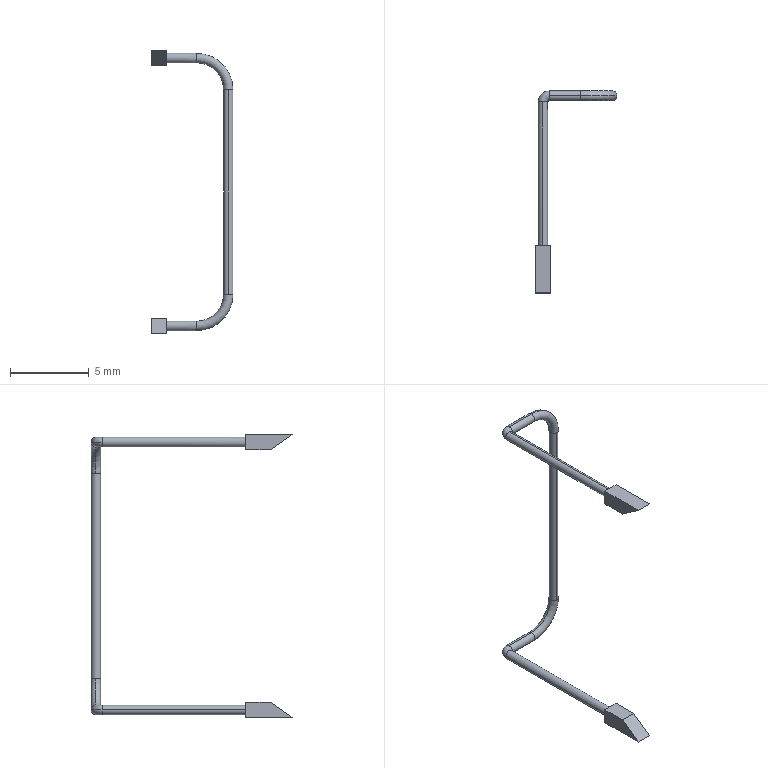Part | SolidWorks | features 3DProfileFeature 2, ICE 2, Sweep 1 | 1 solid | 30 faces | box 5.2 x 12.8 x 18 mm | volume 16.656 mm3 | plane 12 | cylinder 10 | torus 8 | commonest cylinder face diameters 0.6 x10
STEP:
#1=CARTESIAN_POINT('',(0.4,12.5,-16.7));
#2=VERTEX_POINT('',#1);
#3=CARTESIAN_POINT('',(0.4,12.8,-17.));
#4=VERTEX_POINT('',#3);
#5=CARTESIAN_POINT('',(0.4,12.5,-17.));
#6=DIRECTION('',(-1.,0.,0.));
#7=DIRECTION('',(0.,0.,-1.));
#8=AXIS2_PLACEMENT_3D('',#5,#6,#7);
#9=CIRCLE('',#8,0.3);
#10=EDGE_CURVE('',#2,#4,#9,.T.);
#11=ORIENTED_EDGE('',*,*,#10,.T.);
#12=CARTESIAN_POINT('',(-0.3,12.1,-17.));
#13=VERTEX_POINT('',#12);
#14=CARTESIAN_POINT('',(0.4,12.1,-17.));
#15=DIRECTION('',(0.,0.,1.));
#16=DIRECTION('',(1.,0.,0.));
#17=AXIS2_PLACEMENT_3D('',#14,#15,#16);
#18=CIRCLE('',#17,0.7);
#19=EDGE_CURVE('',#4,#13,#18,.T.);
#20=ORIENTED_EDGE('',*,*,#19,.T.);
#21=CARTESIAN_POINT('',(0.3,12.1,-17.));
#22=VERTEX_POINT('',#21);
#23=CARTESIAN_POINT('',(0.,12.1,-17.));
#24=DIRECTION('',(0.,-1.,0.));
#25=DIRECTION('',(0.,0.,-1.));
#26=AXIS2_PLACEMENT_3D('',#23,#24,#25);
#27=CIRCLE('',#26,0.3);
#28=EDGE_CURVE('',#22,#13,#27,.T.);
#29=ORIENTED_EDGE('',*,*,#28,.F.);
#30=CARTESIAN_POINT('',(0.4,12.2,-17.));
#31=VERTEX_POINT('',#30);
#32=CARTESIAN_POINT('',(0.4,12.1,-17.));
#33=DIRECTION('',(0.,0.,1.));
#34=DIRECTION('',(1.,0.,0.));
#35=AXIS2_PLACEMENT_3D('',#32,#33,#34);
#36=CIRCLE('',#35,0.1);
#37=EDGE_CURVE('',#31,#22,#36,.T.);
#38=ORIENTED_EDGE('',*,*,#37,.F.);
#39=CARTESIAN_POINT('',(0.4,12.5,-17.));
#40=DIRECTION('',(-1.,0.,0.));
#41=DIRECTION('',(0.,0.,-1.));
#42=AXIS2_PLACEMENT_3D('',#39,#40,#41);
#43=CIRCLE('',#42,0.3);
#44=EDGE_CURVE('',#31,#2,#43,.T.);
#45=ORIENTED_EDGE('',*,*,#44,.T.);
#46=EDGE_LOOP('',(#11,#20,#29,#38,#45));
#47=FACE_OUTER_BOUND('',#46,.T.);
#48=CARTESIAN_POINT('',(0.4,12.1,-17.));
#49=DIRECTION('',(0.,0.,1.));
#50=DIRECTION('',(1.,0.,0.));
#51=AXIS2_PLACEMENT_3D('',#48,#49,#50);
#52=TOROIDAL_SURFACE('',#51,0.4,0.3);
#53=ADVANCED_FACE('',(#47),#52,.T.);
#54=CARTESIAN_POINT('',(4.4,12.8,-15.));
#55=VERTEX_POINT('',#54);
#56=CARTESIAN_POINT('',(4.7,12.5,-15.));
#57=VERTEX_POINT('',#56);
#58=CARTESIAN_POINT('',(4.4,12.5,-15.));
#59=DIRECTION('',(0.,0.,-1.));
#60=DIRECTION('',(1.,0.,0.));
#61=AXIS2_PLACEMENT_3D('',#58,#59,#60);
#62=CIRCLE('',#61,0.3);
#63=EDGE_CURVE('',#55,#57,#62,.T.);
#64=ORIENTED_EDGE('',*,*,#63,.T.);
#65=CARTESIAN_POINT('',(2.4,12.5,-17.3));
#66=VERTEX_POINT('',#65);
#67=CARTESIAN_POINT('',(2.4,12.5,-15.));
#68=DIRECTION('',(0.,1.,0.));
#69=DIRECTION('',(0.,0.,1.));
#70=AXIS2_PLACEMENT_3D('',#67,#68,#69);
#71=CIRCLE('',#70,2.3);
#72=EDGE_CURVE('',#57,#66,#71,.T.);
#73=ORIENTED_EDGE('',*,*,#72,.T.);
#74=CARTESIAN_POINT('',(2.4,12.5,-16.7));
#75=VERTEX_POINT('',#74);
#76=CARTESIAN_POINT('',(2.4,12.5,-17.));
#77=DIRECTION('',(-1.,0.,0.));
#78=DIRECTION('',(0.,0.,-1.));
#79=AXIS2_PLACEMENT_3D('',#76,#77,#78);
#80=CIRCLE('',#79,0.3);
#81=EDGE_CURVE('',#75,#66,#80,.T.);
#82=ORIENTED_EDGE('',*,*,#81,.F.);
#83=CARTESIAN_POINT('',(4.1,12.5,-15.));
#84=VERTEX_POINT('',#83);
#85=CARTESIAN_POINT('',(2.4,12.5,-15.));
#86=DIRECTION('',(0.,1.,0.));
#87=DIRECTION('',(0.,0.,1.));
#88=AXIS2_PLACEMENT_3D('',#85,#86,#87);
#89=CIRCLE('',#88,1.7);
#90=EDGE_CURVE('',#84,#75,#89,.T.);
#91=ORIENTED_EDGE('',*,*,#90,.F.);
#92=CARTESIAN_POINT('',(4.4,12.5,-15.));
#93=DIRECTION('',(0.,0.,-1.));
#94=DIRECTION('',(1.,0.,0.));
#95=AXIS2_PLACEMENT_3D('',#92,#93,#94);
#96=CIRCLE('',#95,0.3);
#97=EDGE_CURVE('',#84,#55,#96,.T.);
#98=ORIENTED_EDGE('',*,*,#97,.T.);
#99=EDGE_LOOP('',(#64,#73,#82,#91,#98));
#100=FACE_OUTER_BOUND('',#99,.T.);
#101=CARTESIAN_POINT('',(2.4,12.5,-15.));
#102=DIRECTION('',(0.,1.,0.));
#103=DIRECTION('',(0.,0.,1.));
#104=AXIS2_PLACEMENT_3D('',#101,#102,#103);
#105=TOROIDAL_SURFACE('',#104,2.,0.3);
#106=ADVANCED_FACE('',(#100),#105,.T.);
#107=CARTESIAN_POINT('',(2.4,12.5,-0.3));
#108=VERTEX_POINT('',#107);
#109=CARTESIAN_POINT('',(2.4,12.5,0.3));
#110=VERTEX_POINT('',#109);
#111=CARTESIAN_POINT('',(2.4,12.5,0.));
#112=DIRECTION('',(1.,0.,0.));
#113=DIRECTION('',(0.,0.,1.));
#114=AXIS2_PLACEMENT_3D('',#111,#112,#113);
#115=CIRCLE('',#114,0.3);
#116=EDGE_CURVE('',#108,#110,#115,.T.);
#117=ORIENTED_EDGE('',*,*,#116,.T.);
#118=CARTESIAN_POINT('',(4.7,12.5,-2.));
#119=VERTEX_POINT('',#118);
#120=CARTESIAN_POINT('',(2.4,12.5,-2.));
#121=DIRECTION('',(0.,1.,0.));
#122=DIRECTION('',(0.,0.,1.));
#123=AXIS2_PLACEMENT_3D('',#120,#121,#122);
#124=CIRCLE('',#123,2.3);
#125=EDGE_CURVE('',#110,#119,#124,.T.);
#126=ORIENTED_EDGE('',*,*,#125,.T.);
#127=CARTESIAN_POINT('',(4.4,12.8,-2.));
#128=VERTEX_POINT('',#127);
#129=CARTESIAN_POINT('',(4.4,12.5,-2.));
#130=DIRECTION('',(0.,0.,-1.));
#131=DIRECTION('',(1.,0.,0.));
#132=AXIS2_PLACEMENT_3D('',#129,#130,#131);
#133=CIRCLE('',#132,0.3);
#134=EDGE_CURVE('',#128,#119,#133,.T.);
#135=ORIENTED_EDGE('',*,*,#134,.F.);
#136=CARTESIAN_POINT('',(4.1,12.5,-2.));
#137=VERTEX_POINT('',#136);
#138=CARTESIAN_POINT('',(4.4,12.5,-2.));
#139=DIRECTION('',(0.,0.,-1.));
#140=DIRECTION('',(1.,0.,0.));
#141=AXIS2_PLACEMENT_3D('',#138,#139,#140);
#142=CIRCLE('',#141,0.3);
#143=EDGE_CURVE('',#137,#128,#142,.T.);
#144=ORIENTED_EDGE('',*,*,#143,.F.);
#145=CARTESIAN_POINT('',(2.4,12.5,-2.));
#146=DIRECTION('',(0.,1.,0.));
#147=DIRECTION('',(0.,0.,1.));
#148=AXIS2_PLACEMENT_3D('',#145,#146,#147);
#149=CIRCLE('',#148,1.7);
#150=EDGE_CURVE('',#108,#137,#149,.T.);
#151=ORIENTED_EDGE('',*,*,#150,.F.);
#152=EDGE_LOOP('',(#117,#126,#135,#144,#151));
#153=FACE_OUTER_BOUND('',#152,.T.);
#154=CARTESIAN_POINT('',(2.4,12.5,-2.));
#155=DIRECTION('',(0.,1.,0.));
#156=DIRECTION('',(0.,0.,1.));
#157=AXIS2_PLACEMENT_3D('',#154,#155,#156);
#158=TOROIDAL_SURFACE('',#157,2.,0.3);
#159=ADVANCED_FACE('',(#153),#158,.T.);
#160=CARTESIAN_POINT('',(0.,12.1,-0.3));
#161=VERTEX_POINT('',#160);
#162=CARTESIAN_POINT('',(-0.3,12.1,0.));
#163=VERTEX_POINT('',#162);
#164=CARTESIAN_POINT('',(0.,12.1,0.));
#165=DIRECTION('',(0.,1.,0.));
#166=DIRECTION('',(0.,0.,1.));
#167=AXIS2_PLACEMENT_3D('',#164,#165,#166);
#168=CIRCLE('',#167,0.3);
#169=EDGE_CURVE('',#161,#163,#168,.T.);
#170=ORIENTED_EDGE('',*,*,#169,.T.);
#171=CARTESIAN_POINT('',(0.4,12.8,0.));
#172=VERTEX_POINT('',#171);
#173=CARTESIAN_POINT('',(0.4,12.1,0.));
#174=DIRECTION('',(0.,0.,-1.));
#175=DIRECTION('',(-1.,0.,0.));
#176=AXIS2_PLACEMENT_3D('',#173,#174,#175);
#177=CIRCLE('',#176,0.7);
#178=EDGE_CURVE('',#163,#172,#177,.T.);
#179=ORIENTED_EDGE('',*,*,#178,.T.);
#180=CARTESIAN_POINT('',(0.4,12.5,-0.3));
#181=VERTEX_POINT('',#180);
#182=CARTESIAN_POINT('',(0.4,12.5,0.));
#183=DIRECTION('',(1.,0.,0.));
#184=DIRECTION('',(0.,0.,1.));
#185=AXIS2_PLACEMENT_3D('',#182,#183,#184);
#186=CIRCLE('',#185,0.3);
#187=EDGE_CURVE('',#181,#172,#186,.T.);
#188=ORIENTED_EDGE('',*,*,#187,.F.);
#189=CARTESIAN_POINT('',(0.4,12.2,0.));
#190=VERTEX_POINT('',#189);
#191=CARTESIAN_POINT('',(0.4,12.5,0.));
#192=DIRECTION('',(1.,0.,0.));
#193=DIRECTION('',(0.,0.,1.));
#194=AXIS2_PLACEMENT_3D('',#191,#192,#193);
#195=CIRCLE('',#194,0.3);
#196=EDGE_CURVE('',#190,#181,#195,.T.);
#197=ORIENTED_EDGE('',*,*,#196,.F.);
#198=CARTESIAN_POINT('',(0.3,12.1,0.));
#199=VERTEX_POINT('',#198);
#200=CARTESIAN_POINT('',(0.4,12.1,0.));
#201=DIRECTION('',(0.,0.,-1.));
#202=DIRECTION('',(-1.,0.,0.));
#203=AXIS2_PLACEMENT_3D('',#200,#201,#202);
#204=CIRCLE('',#203,0.1);
#205=EDGE_CURVE('',#199,#190,#204,.T.);
#206=ORIENTED_EDGE('',*,*,#205,.F.);
#207=CARTESIAN_POINT('',(0.,12.1,0.));
#208=DIRECTION('',(0.,1.,0.));
#209=DIRECTION('',(0.,0.,1.));
#210=AXIS2_PLACEMENT_3D('',#207,#208,#209);
#211=CIRCLE('',#210,0.3);
#212=EDGE_CURVE('',#199,#161,#211,.T.);
#213=ORIENTED_EDGE('',*,*,#212,.T.);
#214=EDGE_LOOP('',(#170,#179,#188,#197,#206,#213));
#215=FACE_OUTER_BOUND('',#214,.T.);
#216=CARTESIAN_POINT('',(0.4,12.1,0.));
#217=DIRECTION('',(0.,0.,-1.));
#218=DIRECTION('',(-1.,0.,0.));
#219=AXIS2_PLACEMENT_3D('',#216,#217,#218);
#220=TOROIDAL_SURFACE('',#219,0.4,0.3);
#221=ADVANCED_FACE('',(#215),#220,.T.);
#222=ORIENTED_EDGE('',*,*,#28,.T.);
#223=CARTESIAN_POINT('',(-0.3,3.,-17.));
#224=VERTEX_POINT('',#223);
#225=CARTESIAN_POINT('',(-0.3,12.1,-17.));
#226=DIRECTION('',(0.,-1.,0.));
#227=VECTOR('',#226,1000.);
#228=LINE('',#225,#227);
#229=EDGE_CURVE('',#13,#224,#228,.T.);
#230=ORIENTED_EDGE('',*,*,#229,.T.);
#231=CARTESIAN_POINT('',(0.3,3.,-17.));
#232=VERTEX_POINT('',#231);
#233=CARTESIAN_POINT('',(0.,3.,-17.));
#234=DIRECTION('',(0.,-1.,0.));
#235=DIRECTION('',(0.,0.,1.));
#236=AXIS2_PLACEMENT_3D('',#233,#234,#235);
#237=CIRCLE('',#236,0.3);
#238=EDGE_CURVE('',#232,#224,#237,.T.);
#239=ORIENTED_EDGE('',*,*,#238,.F.);
#240=CARTESIAN_POINT('',(0.3,12.1,-17.));
#241=DIRECTION('',(0.,-1.,0.));
#242=VECTOR('',#241,1000.);
#243=LINE('',#240,#242);
#244=EDGE_CURVE('',#22,#232,#243,.T.);
#245=ORIENTED_EDGE('',*,*,#244,.F.);
#246=EDGE_LOOP('',(#222,#230,#239,#245));
#247=FACE_OUTER_BOUND('',#246,.T.);
#248=CARTESIAN_POINT('',(0.,12.1,-17.));
#249=DIRECTION('',(0.,-1.,0.));
#250=DIRECTION('',(1.,0.,0.));
#251=AXIS2_PLACEMENT_3D('',#248,#249,#250);
#252=CYLINDRICAL_SURFACE('',#251,0.3);
#253=ADVANCED_FACE('',(#247),#252,.T.);
#254=ORIENTED_EDGE('',*,*,#81,.T.);
#255=CARTESIAN_POINT('',(0.4,12.5,-17.3));
#256=VERTEX_POINT('',#255);
#257=CARTESIAN_POINT('',(2.4,12.5,-17.3));
#258=DIRECTION('',(-1.,0.,0.));
#259=VECTOR('',#258,1000.);
#260=LINE('',#257,#259);
#261=EDGE_CURVE('',#66,#256,#260,.T.);
#262=ORIENTED_EDGE('',*,*,#261,.T.);
#263=CARTESIAN_POINT('',(0.4,12.5,-17.));
#264=DIRECTION('',(-1.,0.,0.));
#265=DIRECTION('',(0.,0.,-1.));
#266=AXIS2_PLACEMENT_3D('',#263,#264,#265);
#267=CIRCLE('',#266,0.3);
#268=EDGE_CURVE('',#4,#256,#267,.T.);
#269=ORIENTED_EDGE('',*,*,#268,.F.);
#270=ORIENTED_EDGE('',*,*,#10,.F.);
#271=CARTESIAN_POINT('',(2.4,12.5,-16.7));
#272=DIRECTION('',(-1.,0.,0.));
#273=VECTOR('',#272,1000.);
#274=LINE('',#271,#273);
#275=EDGE_CURVE('',#75,#2,#274,.T.);
#276=ORIENTED_EDGE('',*,*,#275,.F.);
#277=EDGE_LOOP('',(#254,#262,#269,#270,#276));
#278=FACE_OUTER_BOUND('',#277,.T.);
#279=CARTESIAN_POINT('',(2.4,12.5,-17.));
#280=DIRECTION('',(-1.,0.,0.));
#281=DIRECTION('',(0.,0.,1.));
#282=AXIS2_PLACEMENT_3D('',#279,#280,#281);
#283=CYLINDRICAL_SURFACE('',#282,0.3);
#284=ADVANCED_FACE('',(#278),#283,.T.);
#285=ORIENTED_EDGE('',*,*,#134,.T.);
#286=CARTESIAN_POINT('',(4.4,12.2,-2.));
#287=VERTEX_POINT('',#286);
#288=CARTESIAN_POINT('',(4.4,12.5,-2.));
#289=DIRECTION('',(0.,0.,-1.));
#290=DIRECTION('',(1.,0.,0.));
#291=AXIS2_PLACEMENT_3D('',#288,#289,#290);
#292=CIRCLE('',#291,0.3);
#293=EDGE_CURVE('',#119,#287,#292,.T.);
#294=ORIENTED_EDGE('',*,*,#293,.T.);
#295=CARTESIAN_POINT('',(4.4,12.2,-15.));
#296=VERTEX_POINT('',#295);
#297=CARTESIAN_POINT('',(4.4,12.2,-2.));
#298=DIRECTION('',(0.,0.,-1.));
#299=VECTOR('',#298,1000.);
#300=LINE('',#297,#299);
#301=EDGE_CURVE('',#287,#296,#300,.T.);
#302=ORIENTED_EDGE('',*,*,#301,.T.);
#303=CARTESIAN_POINT('',(4.4,12.5,-15.));
#304=DIRECTION('',(0.,0.,-1.));
#305=DIRECTION('',(1.,0.,0.));
#306=AXIS2_PLACEMENT_3D('',#303,#304,#305);
#307=CIRCLE('',#306,0.3);
#308=EDGE_CURVE('',#57,#296,#307,.T.);
#309=ORIENTED_EDGE('',*,*,#308,.F.);
#310=ORIENTED_EDGE('',*,*,#63,.F.);
#311=CARTESIAN_POINT('',(4.4,12.8,-2.));
#312=DIRECTION('',(0.,0.,-1.));
#313=VECTOR('',#312,1000.);
#314=LINE('',#311,#313);
#315=EDGE_CURVE('',#128,#55,#314,.T.);
#316=ORIENTED_EDGE('',*,*,#315,.F.);
#317=EDGE_LOOP('',(#285,#294,#302,#309,#310,#316));
#318=FACE_OUTER_BOUND('',#317,.T.);
#319=CARTESIAN_POINT('',(4.4,12.5,-2.));
#320=DIRECTION('',(0.,0.,-1.));
#321=DIRECTION('',(0.,1.,0.));
#322=AXIS2_PLACEMENT_3D('',#319,#320,#321);
#323=CYLINDRICAL_SURFACE('',#322,0.3);
#324=ADVANCED_FACE('',(#318),#323,.T.);
#325=ORIENTED_EDGE('',*,*,#187,.T.);
#326=CARTESIAN_POINT('',(0.4,12.5,0.3));
#327=VERTEX_POINT('',#326);
#328=CARTESIAN_POINT('',(0.4,12.5,0.));
#329=DIRECTION('',(1.,0.,0.));
#330=DIRECTION('',(0.,0.,1.));
#331=AXIS2_PLACEMENT_3D('',#328,#329,#330);
#332=CIRCLE('',#331,0.3);
#333=EDGE_CURVE('',#172,#327,#332,.T.);
#334=ORIENTED_EDGE('',*,*,#333,.T.);
#335=CARTESIAN_POINT('',(0.4,12.5,0.3));
#336=DIRECTION('',(1.,0.,0.));
#337=VECTOR('',#336,1000.);
#338=LINE('',#335,#337);
#339=EDGE_CURVE('',#327,#110,#338,.T.);
#340=ORIENTED_EDGE('',*,*,#339,.T.);
#341=ORIENTED_EDGE('',*,*,#116,.F.);
#342=CARTESIAN_POINT('',(0.4,12.5,-0.3));
#343=DIRECTION('',(1.,0.,0.));
#344=VECTOR('',#343,1000.);
#345=LINE('',#342,#344);
#346=EDGE_CURVE('',#181,#108,#345,.T.);
#347=ORIENTED_EDGE('',*,*,#346,.F.);
#348=EDGE_LOOP('',(#325,#334,#340,#341,#347));
#349=FACE_OUTER_BOUND('',#348,.T.);
#350=CARTESIAN_POINT('',(0.4,12.5,0.));
#351=DIRECTION('',(1.,0.,0.));
#352=DIRECTION('',(0.,0.,-1.));
#353=AXIS2_PLACEMENT_3D('',#350,#351,#352);
#354=CYLINDRICAL_SURFACE('',#353,0.3);
#355=ADVANCED_FACE('',(#349),#354,.T.);
#356=CARTESIAN_POINT('',(0.,3.,-0.3));
#357=VERTEX_POINT('',#356);
#358=CARTESIAN_POINT('',(0.,3.,0.3));
#359=VERTEX_POINT('',#358);
#360=CARTESIAN_POINT('',(0.,3.,0.));
#361=DIRECTION('',(0.,-1.,0.));
#362=DIRECTION('',(0.,0.,1.));
#363=AXIS2_PLACEMENT_3D('',#360,#361,#362);
#364=CIRCLE('',#363,0.3);
#365=EDGE_CURVE('',#357,#359,#364,.T.);
#366=ORIENTED_EDGE('',*,*,#365,.F.);
#367=CARTESIAN_POINT('',(0.,0.,-0.3));
#368=DIRECTION('',(0.,1.,0.));
#369=VECTOR('',#368,1000.);
#370=LINE('',#367,#369);
#371=EDGE_CURVE('',#357,#161,#370,.T.);
#372=ORIENTED_EDGE('',*,*,#371,.T.);
#373=ORIENTED_EDGE('',*,*,#212,.F.);
#374=CARTESIAN_POINT('',(0.,12.1,0.3));
#375=VERTEX_POINT('',#374);
#376=CARTESIAN_POINT('',(0.,12.1,0.));
#377=DIRECTION('',(0.,1.,0.));
#378=DIRECTION('',(0.,0.,1.));
#379=AXIS2_PLACEMENT_3D('',#376,#377,#378);
#380=CIRCLE('',#379,0.3);
#381=EDGE_CURVE('',#375,#199,#380,.T.);
#382=ORIENTED_EDGE('',*,*,#381,.F.);
#383=CARTESIAN_POINT('',(0.,0.,0.3));
#384=DIRECTION('',(0.,1.,0.));
#385=VECTOR('',#384,1000.);
#386=LINE('',#383,#385);
#387=EDGE_CURVE('',#359,#375,#386,.T.);
#388=ORIENTED_EDGE('',*,*,#387,.F.);
#389=EDGE_LOOP('',(#366,#372,#373,#382,#388));
#390=FACE_OUTER_BOUND('',#389,.T.);
#391=CARTESIAN_POINT('',(0.,0.,0.));
#392=DIRECTION('',(0.,1.,0.));
#393=DIRECTION('',(0.,0.,1.));
#394=AXIS2_PLACEMENT_3D('',#391,#392,#393);
#395=CYLINDRICAL_SURFACE('',#394,0.3);
#396=ADVANCED_FACE('',(#390),#395,.T.);
#397=ORIENTED_EDGE('',*,*,#229,.F.);
#398=CARTESIAN_POINT('',(0.,12.1,-17.));
#399=DIRECTION('',(0.,-1.,0.));
#400=DIRECTION('',(0.,0.,-1.));
#401=AXIS2_PLACEMENT_3D('',#398,#399,#400);
#402=CIRCLE('',#401,0.3);
#403=EDGE_CURVE('',#13,#22,#402,.T.);
#404=ORIENTED_EDGE('',*,*,#403,.T.);
#405=ORIENTED_EDGE('',*,*,#244,.T.);
#406=CARTESIAN_POINT('',(0.,3.,-17.));
#407=DIRECTION('',(0.,-1.,0.));
#408=DIRECTION('',(0.,0.,1.));
#409=AXIS2_PLACEMENT_3D('',#406,#407,#408);
#410=CIRCLE('',#409,0.3);
#411=EDGE_CURVE('',#224,#232,#410,.T.);
#412=ORIENTED_EDGE('',*,*,#411,.F.);
#413=EDGE_LOOP('',(#397,#404,#405,#412));
#414=FACE_OUTER_BOUND('',#413,.T.);
#415=CARTESIAN_POINT('',(0.,12.1,-17.));
#416=DIRECTION('',(0.,-1.,0.));
#417=DIRECTION('',(1.,0.,0.));
#418=AXIS2_PLACEMENT_3D('',#415,#416,#417);
#419=CYLINDRICAL_SURFACE('',#418,0.3);
#420=ADVANCED_FACE('',(#414),#419,.T.);
#421=ORIENTED_EDGE('',*,*,#19,.F.);
#422=ORIENTED_EDGE('',*,*,#268,.T.);
#423=CARTESIAN_POINT('',(0.4,12.5,-17.));
#424=DIRECTION('',(-1.,0.,0.));
#425=DIRECTION('',(0.,0.,-1.));
#426=AXIS2_PLACEMENT_3D('',#423,#424,#425);
#427=CIRCLE('',#426,0.3);
#428=EDGE_CURVE('',#256,#31,#427,.T.);
#429=ORIENTED_EDGE('',*,*,#428,.T.);
#430=ORIENTED_EDGE('',*,*,#37,.T.);
#431=ORIENTED_EDGE('',*,*,#403,.F.);
#432=EDGE_LOOP('',(#421,#422,#429,#430,#431));
#433=FACE_OUTER_BOUND('',#432,.T.);
#434=CARTESIAN_POINT('',(0.4,12.1,-17.));
#435=DIRECTION('',(0.,0.,1.));
#436=DIRECTION('',(1.,0.,0.));
#437=AXIS2_PLACEMENT_3D('',#434,#435,#436);
#438=TOROIDAL_SURFACE('',#437,0.4,0.3);
#439=ADVANCED_FACE('',(#433),#438,.T.);
#440=ORIENTED_EDGE('',*,*,#261,.F.);
#441=CARTESIAN_POINT('',(2.4,12.5,-17.));
#442=DIRECTION('',(-1.,0.,0.));
#443=DIRECTION('',(0.,0.,-1.));
#444=AXIS2_PLACEMENT_3D('',#441,#442,#443);
#445=CIRCLE('',#444,0.3);
#446=EDGE_CURVE('',#66,#75,#445,.T.);
#447=ORIENTED_EDGE('',*,*,#446,.T.);
#448=ORIENTED_EDGE('',*,*,#275,.T.);
#449=ORIENTED_EDGE('',*,*,#44,.F.);
#450=ORIENTED_EDGE('',*,*,#428,.F.);
#451=EDGE_LOOP('',(#440,#447,#448,#449,#450));
#452=FACE_OUTER_BOUND('',#451,.T.);
#453=CARTESIAN_POINT('',(2.4,12.5,-17.));
#454=DIRECTION('',(-1.,0.,0.));
#455=DIRECTION('',(0.,0.,1.));
#456=AXIS2_PLACEMENT_3D('',#453,#454,#455);
#457=CYLINDRICAL_SURFACE('',#456,0.3);
#458=ADVANCED_FACE('',(#452),#457,.T.);
#459=ORIENTED_EDGE('',*,*,#72,.F.);
#460=ORIENTED_EDGE('',*,*,#308,.T.);
#461=CARTESIAN_POINT('',(4.4,12.5,-15.));
#462=DIRECTION('',(0.,0.,-1.));
#463=DIRECTION('',(1.,0.,0.));
#464=AXIS2_PLACEMENT_3D('',#461,#462,#463);
#465=CIRCLE('',#464,0.3);
#466=EDGE_CURVE('',#296,#84,#465,.T.);
#467=ORIENTED_EDGE('',*,*,#466,.T.);
#468=ORIENTED_EDGE('',*,*,#90,.T.);
#469=ORIENTED_EDGE('',*,*,#446,.F.);
#470=EDGE_LOOP('',(#459,#460,#467,#468,#469));
#471=FACE_OUTER_BOUND('',#470,.T.);
#472=CARTESIAN_POINT('',(2.4,12.5,-15.));
#473=DIRECTION('',(0.,1.,0.));
#474=DIRECTION('',(0.,0.,1.));
#475=AXIS2_PLACEMENT_3D('',#472,#473,#474);
#476=TOROIDAL_SURFACE('',#475,2.,0.3);
#477=ADVANCED_FACE('',(#471),#476,.T.);
#478=ORIENTED_EDGE('',*,*,#301,.F.);
#479=CARTESIAN_POINT('',(4.4,12.5,-2.));
#480=DIRECTION('',(0.,0.,-1.));
#481=DIRECTION('',(1.,0.,0.));
#482=AXIS2_PLACEMENT_3D('',#479,#480,#481);
#483=CIRCLE('',#482,0.3);
#484=EDGE_CURVE('',#287,#137,#483,.T.);
#485=ORIENTED_EDGE('',*,*,#484,.T.);
#486=ORIENTED_EDGE('',*,*,#143,.T.);
#487=ORIENTED_EDGE('',*,*,#315,.T.);
#488=ORIENTED_EDGE('',*,*,#97,.F.);
#489=ORIENTED_EDGE('',*,*,#466,.F.);
#490=EDGE_LOOP('',(#478,#485,#486,#487,#488,#489));
#491=FACE_OUTER_BOUND('',#490,.T.);
#492=CARTESIAN_POINT('',(4.4,12.5,-2.));
#493=DIRECTION('',(0.,0.,-1.));
#494=DIRECTION('',(0.,1.,0.));
#495=AXIS2_PLACEMENT_3D('',#492,#493,#494);
#496=CYLINDRICAL_SURFACE('',#495,0.3);
#497=ADVANCED_FACE('',(#491),#496,.T.);
#498=ORIENTED_EDGE('',*,*,#125,.F.);
#499=CARTESIAN_POINT('',(2.4,12.5,0.));
#500=DIRECTION('',(1.,0.,0.));
#501=DIRECTION('',(0.,0.,1.));
#502=AXIS2_PLACEMENT_3D('',#499,#500,#501);
#503=CIRCLE('',#502,0.3);
#504=EDGE_CURVE('',#110,#108,#503,.T.);
#505=ORIENTED_EDGE('',*,*,#504,.T.);
#506=ORIENTED_EDGE('',*,*,#150,.T.);
#507=ORIENTED_EDGE('',*,*,#484,.F.);
#508=ORIENTED_EDGE('',*,*,#293,.F.);
#509=EDGE_LOOP('',(#498,#505,#506,#507,#508));
#510=FACE_OUTER_BOUND('',#509,.T.);
#511=CARTESIAN_POINT('',(2.4,12.5,-2.));
#512=DIRECTION('',(0.,1.,0.));
#513=DIRECTION('',(0.,0.,1.));
#514=AXIS2_PLACEMENT_3D('',#511,#512,#513);
#515=TOROIDAL_SURFACE('',#514,2.,0.3);
#516=ADVANCED_FACE('',(#510),#515,.T.);
#517=ORIENTED_EDGE('',*,*,#339,.F.);
#518=CARTESIAN_POINT('',(0.4,12.5,0.));
#519=DIRECTION('',(1.,0.,0.));
#520=DIRECTION('',(0.,0.,1.));
#521=AXIS2_PLACEMENT_3D('',#518,#519,#520);
#522=CIRCLE('',#521,0.3);
#523=EDGE_CURVE('',#327,#190,#522,.T.);
#524=ORIENTED_EDGE('',*,*,#523,.T.);
#525=ORIENTED_EDGE('',*,*,#196,.T.);
#526=ORIENTED_EDGE('',*,*,#346,.T.);
#527=ORIENTED_EDGE('',*,*,#504,.F.);
#528=EDGE_LOOP('',(#517,#524,#525,#526,#527));
#529=FACE_OUTER_BOUND('',#528,.T.);
#530=CARTESIAN_POINT('',(0.4,12.5,0.));
#531=DIRECTION('',(1.,0.,0.));
#532=DIRECTION('',(0.,0.,-1.));
#533=AXIS2_PLACEMENT_3D('',#530,#531,#532);
#534=CYLINDRICAL_SURFACE('',#533,0.3);
#535=ADVANCED_FACE('',(#529),#534,.T.);
#536=ORIENTED_EDGE('',*,*,#178,.F.);
#537=CARTESIAN_POINT('',(0.,12.1,0.));
#538=DIRECTION('',(0.,1.,0.));
#539=DIRECTION('',(0.,0.,1.));
#540=AXIS2_PLACEMENT_3D('',#537,#538,#539);
#541=CIRCLE('',#540,0.3);
#542=EDGE_CURVE('',#163,#375,#541,.T.);
#543=ORIENTED_EDGE('',*,*,#542,.T.);
#544=ORIENTED_EDGE('',*,*,#381,.T.);
#545=ORIENTED_EDGE('',*,*,#205,.T.);
#546=ORIENTED_EDGE('',*,*,#523,.F.);
#547=ORIENTED_EDGE('',*,*,#333,.F.);
#548=EDGE_LOOP('',(#536,#543,#544,#545,#546,#547));
#549=FACE_OUTER_BOUND('',#548,.T.);
#550=CARTESIAN_POINT('',(0.4,12.1,0.));
#551=DIRECTION('',(0.,0.,-1.));
#552=DIRECTION('',(-1.,0.,0.));
#553=AXIS2_PLACEMENT_3D('',#550,#551,#552);
#554=TOROIDAL_SURFACE('',#553,0.4,0.3);
#555=ADVANCED_FACE('',(#549),#554,.T.);
#556=ORIENTED_EDGE('',*,*,#371,.F.);
#557=CARTESIAN_POINT('',(0.,3.,0.));
#558=DIRECTION('',(0.,-1.,0.));
#559=DIRECTION('',(0.,0.,1.));
#560=AXIS2_PLACEMENT_3D('',#557,#558,#559);
#561=CIRCLE('',#560,0.3);
#562=EDGE_CURVE('',#359,#357,#561,.T.);
#563=ORIENTED_EDGE('',*,*,#562,.F.);
#564=ORIENTED_EDGE('',*,*,#387,.T.);
#565=ORIENTED_EDGE('',*,*,#542,.F.);
#566=ORIENTED_EDGE('',*,*,#169,.F.);
#567=EDGE_LOOP('',(#556,#563,#564,#565,#566));
#568=FACE_OUTER_BOUND('',#567,.T.);
#569=CARTESIAN_POINT('',(0.,0.,0.));
#570=DIRECTION('',(0.,1.,0.));
#571=DIRECTION('',(0.,0.,1.));
#572=AXIS2_PLACEMENT_3D('',#569,#570,#571);
#573=CYLINDRICAL_SURFACE('',#572,0.3);
#574=ADVANCED_FACE('',(#568),#573,.T.);
#575=CARTESIAN_POINT('',(-0.5,0.,-17.5));
#576=VERTEX_POINT('',#575);
#577=CARTESIAN_POINT('',(-0.5,1.428,-16.5));
#578=VERTEX_POINT('',#577);
#579=CARTESIAN_POINT('',(-0.5,2.947,-15.437));
#580=DIRECTION('',(0.,0.8192,0.5736));
#581=VECTOR('',#580,1000.);
#582=LINE('',#579,#581);
#583=EDGE_CURVE('',#576,#578,#582,.T.);
#584=ORIENTED_EDGE('',*,*,#583,.T.);
#585=CARTESIAN_POINT('',(-0.5,3.,-16.5));
#586=VERTEX_POINT('',#585);
#587=CARTESIAN_POINT('',(-0.5,3.,-16.5));
#588=DIRECTION('',(0.,-1.,0.));
#589=VECTOR('',#588,1000.);
#590=LINE('',#587,#589);
#591=EDGE_CURVE('',#586,#578,#590,.T.);
#592=ORIENTED_EDGE('',*,*,#591,.F.);
#593=CARTESIAN_POINT('',(-0.5,3.,-17.5));
#594=VERTEX_POINT('',#593);
#595=CARTESIAN_POINT('',(-0.5,3.,-16.5));
#596=DIRECTION('',(0.,0.,-1.));
#597=VECTOR('',#596,1000.);
#598=LINE('',#595,#597);
#599=EDGE_CURVE('',#586,#594,#598,.T.);
#600=ORIENTED_EDGE('',*,*,#599,.T.);
#601=CARTESIAN_POINT('',(-0.5,3.,-17.5));
#602=DIRECTION('',(0.,-1.,0.));
#603=VECTOR('',#602,1000.);
#604=LINE('',#601,#603);
#605=EDGE_CURVE('',#594,#576,#604,.T.);
#606=ORIENTED_EDGE('',*,*,#605,.T.);
#607=EDGE_LOOP('',(#584,#592,#600,#606));
#608=FACE_OUTER_BOUND('',#607,.T.);
#609=CARTESIAN_POINT('',(-0.5,3.,-16.5));
#610=DIRECTION('',(-1.,0.,0.));
#611=DIRECTION('',(0.,0.,1.));
#612=AXIS2_PLACEMENT_3D('',#609,#610,#611);
#613=PLANE('',#612);
#614=ADVANCED_FACE('',(#608),#613,.T.);
#615=CARTESIAN_POINT('',(0.5,1.428,-16.5));
#616=VERTEX_POINT('',#615);
#617=CARTESIAN_POINT('',(0.5,1.428,-16.5));
#618=DIRECTION('',(-1.,0.,0.));
#619=VECTOR('',#618,1000.);
#620=LINE('',#617,#619);
#621=EDGE_CURVE('',#616,#578,#620,.T.);
#622=ORIENTED_EDGE('',*,*,#621,.F.);
#623=CARTESIAN_POINT('',(0.5,3.,-16.5));
#624=VERTEX_POINT('',#623);
#625=CARTESIAN_POINT('',(0.5,3.,-16.5));
#626=DIRECTION('',(0.,-1.,0.));
#627=VECTOR('',#626,1000.);
#628=LINE('',#625,#627);
#629=EDGE_CURVE('',#624,#616,#628,.T.);
#630=ORIENTED_EDGE('',*,*,#629,.F.);
#631=CARTESIAN_POINT('',(0.5,3.,-16.5));
#632=DIRECTION('',(-1.,0.,0.));
#633=VECTOR('',#632,1000.);
#634=LINE('',#631,#633);
#635=EDGE_CURVE('',#624,#586,#634,.T.);
#636=ORIENTED_EDGE('',*,*,#635,.T.);
#637=ORIENTED_EDGE('',*,*,#591,.T.);
#638=EDGE_LOOP('',(#622,#630,#636,#637));
#639=FACE_OUTER_BOUND('',#638,.T.);
#640=CARTESIAN_POINT('',(0.5,3.,-16.5));
#641=DIRECTION('',(0.,0.,1.));
#642=DIRECTION('',(1.,0.,0.));
#643=AXIS2_PLACEMENT_3D('',#640,#641,#642);
#644=PLANE('',#643);
#645=ADVANCED_FACE('',(#639),#644,.T.);
#646=CARTESIAN_POINT('',(0.5,0.,-17.5));
#647=VERTEX_POINT('',#646);
#648=CARTESIAN_POINT('',(0.5,2.483,-15.761));
#649=DIRECTION('',(0.,0.8192,0.5736));
#650=VECTOR('',#649,1000.);
#651=LINE('',#648,#650);
#652=EDGE_CURVE('',#647,#616,#651,.T.);
#653=ORIENTED_EDGE('',*,*,#652,.F.);
#654=CARTESIAN_POINT('',(0.5,3.,-17.5));
#655=VERTEX_POINT('',#654);
#656=CARTESIAN_POINT('',(0.5,3.,-17.5));
#657=DIRECTION('',(0.,-1.,0.));
#658=VECTOR('',#657,1000.);
#659=LINE('',#656,#658);
#660=EDGE_CURVE('',#655,#647,#659,.T.);
#661=ORIENTED_EDGE('',*,*,#660,.F.);
#662=CARTESIAN_POINT('',(0.5,3.,-16.5));
#663=DIRECTION('',(0.,0.,1.));
#664=VECTOR('',#663,1000.);
#665=LINE('',#662,#664);
#666=EDGE_CURVE('',#655,#624,#665,.T.);
#667=ORIENTED_EDGE('',*,*,#666,.T.);
#668=ORIENTED_EDGE('',*,*,#629,.T.);
#669=EDGE_LOOP('',(#653,#661,#667,#668));
#670=FACE_OUTER_BOUND('',#669,.T.);
#671=CARTESIAN_POINT('',(0.5,3.,-16.5));
#672=DIRECTION('',(1.,0.,0.));
#673=DIRECTION('',(0.,0.,-1.));
#674=AXIS2_PLACEMENT_3D('',#671,#672,#673);
#675=PLANE('',#674);
#676=ADVANCED_FACE('',(#670),#675,.T.);
#677=CARTESIAN_POINT('',(0.5,0.,-17.5));
#678=DIRECTION('',(1.,0.,0.));
#679=VECTOR('',#678,1000.);
#680=LINE('',#677,#679);
#681=EDGE_CURVE('',#576,#647,#680,.T.);
#682=ORIENTED_EDGE('',*,*,#681,.F.);
#683=ORIENTED_EDGE('',*,*,#605,.F.);
#684=CARTESIAN_POINT('',(0.5,3.,-17.5));
#685=DIRECTION('',(1.,0.,0.));
#686=VECTOR('',#685,1000.);
#687=LINE('',#684,#686);
#688=EDGE_CURVE('',#594,#655,#687,.T.);
#689=ORIENTED_EDGE('',*,*,#688,.T.);
#690=ORIENTED_EDGE('',*,*,#660,.T.);
#691=EDGE_LOOP('',(#682,#683,#689,#690));
#692=FACE_OUTER_BOUND('',#691,.T.);
#693=CARTESIAN_POINT('',(0.5,3.,-17.5));
#694=DIRECTION('',(0.,0.,-1.));
#695=DIRECTION('',(-1.,0.,0.));
#696=AXIS2_PLACEMENT_3D('',#693,#694,#695);
#697=PLANE('',#696);
#698=ADVANCED_FACE('',(#692),#697,.T.);
#699=ORIENTED_EDGE('',*,*,#238,.T.);
#700=ORIENTED_EDGE('',*,*,#411,.T.);
#701=EDGE_LOOP('',(#699,#700));
#702=FACE_BOUND('',#701,.T.);
#703=ORIENTED_EDGE('',*,*,#599,.F.);
#704=ORIENTED_EDGE('',*,*,#635,.F.);
#705=ORIENTED_EDGE('',*,*,#666,.F.);
#706=ORIENTED_EDGE('',*,*,#688,.F.);
#707=EDGE_LOOP('',(#703,#704,#705,#706));
#708=FACE_OUTER_BOUND('',#707,.T.);
#709=CARTESIAN_POINT('',(0.,3.,0.));
#710=DIRECTION('',(0.,1.,0.));
#711=DIRECTION('',(0.,0.,1.));
#712=AXIS2_PLACEMENT_3D('',#709,#710,#711);
#713=PLANE('',#712);
#714=ADVANCED_FACE('',(#702,#708),#713,.T.);
#715=CARTESIAN_POINT('',(-0.5,1.428,-0.5));
#716=VERTEX_POINT('',#715);
#717=CARTESIAN_POINT('',(-0.5,0.,0.5));
#718=VERTEX_POINT('',#717);
#719=CARTESIAN_POINT('',(-0.5,0.,0.5));
#720=DIRECTION('',(0.,-0.8192,0.5736));
#721=VECTOR('',#720,1000.);
#722=LINE('',#719,#721);
#723=EDGE_CURVE('',#716,#718,#722,.T.);
#724=ORIENTED_EDGE('',*,*,#723,.T.);
#725=CARTESIAN_POINT('',(-0.5,3.,0.5));
#726=VERTEX_POINT('',#725);
#727=CARTESIAN_POINT('',(-0.5,3.,0.5));
#728=DIRECTION('',(0.,-1.,0.));
#729=VECTOR('',#728,1000.);
#730=LINE('',#727,#729);
#731=EDGE_CURVE('',#726,#718,#730,.T.);
#732=ORIENTED_EDGE('',*,*,#731,.F.);
#733=CARTESIAN_POINT('',(-0.5,3.,-0.5));
#734=VERTEX_POINT('',#733);
#735=CARTESIAN_POINT('',(-0.5,3.,0.5));
#736=DIRECTION('',(0.,0.,-1.));
#737=VECTOR('',#736,1000.);
#738=LINE('',#735,#737);
#739=EDGE_CURVE('',#726,#734,#738,.T.);
#740=ORIENTED_EDGE('',*,*,#739,.T.);
#741=CARTESIAN_POINT('',(-0.5,3.,-0.5));
#742=DIRECTION('',(0.,-1.,0.));
#743=VECTOR('',#742,1000.);
#744=LINE('',#741,#743);
#745=EDGE_CURVE('',#734,#716,#744,.T.);
#746=ORIENTED_EDGE('',*,*,#745,.T.);
#747=EDGE_LOOP('',(#724,#732,#740,#746));
#748=FACE_OUTER_BOUND('',#747,.T.);
#749=CARTESIAN_POINT('',(-0.5,3.,0.5));
#750=DIRECTION('',(-1.,0.,0.));
#751=DIRECTION('',(0.,0.,1.));
#752=AXIS2_PLACEMENT_3D('',#749,#750,#751);
#753=PLANE('',#752);
#754=ADVANCED_FACE('',(#748),#753,.T.);
#755=CARTESIAN_POINT('',(0.5,0.,0.5));
#756=VERTEX_POINT('',#755);
#757=CARTESIAN_POINT('',(0.5,0.,0.5));
#758=DIRECTION('',(-1.,0.,0.));
#759=VECTOR('',#758,1000.);
#760=LINE('',#757,#759);
#761=EDGE_CURVE('',#756,#718,#760,.T.);
#762=ORIENTED_EDGE('',*,*,#761,.F.);
#763=CARTESIAN_POINT('',(0.5,3.,0.5));
#764=VERTEX_POINT('',#763);
#765=CARTESIAN_POINT('',(0.5,3.,0.5));
#766=DIRECTION('',(0.,-1.,0.));
#767=VECTOR('',#766,1000.);
#768=LINE('',#765,#767);
#769=EDGE_CURVE('',#764,#756,#768,.T.);
#770=ORIENTED_EDGE('',*,*,#769,.F.);
#771=CARTESIAN_POINT('',(0.5,3.,0.5));
#772=DIRECTION('',(-1.,0.,0.));
#773=VECTOR('',#772,1000.);
#774=LINE('',#771,#773);
#775=EDGE_CURVE('',#764,#726,#774,.T.);
#776=ORIENTED_EDGE('',*,*,#775,.T.);
#777=ORIENTED_EDGE('',*,*,#731,.T.);
#778=EDGE_LOOP('',(#762,#770,#776,#777));
#779=FACE_OUTER_BOUND('',#778,.T.);
#780=CARTESIAN_POINT('',(0.5,3.,0.5));
#781=DIRECTION('',(0.,0.,1.));
#782=DIRECTION('',(1.,0.,0.));
#783=AXIS2_PLACEMENT_3D('',#780,#781,#782);
#784=PLANE('',#783);
#785=ADVANCED_FACE('',(#779),#784,.T.);
#786=CARTESIAN_POINT('',(0.5,1.428,-0.5));
#787=VERTEX_POINT('',#786);
#788=CARTESIAN_POINT('',(0.5,2.013,-0.9095));
#789=DIRECTION('',(0.,-0.8192,0.5736));
#790=VECTOR('',#789,1000.);
#791=LINE('',#788,#790);
#792=EDGE_CURVE('',#787,#756,#791,.T.);
#793=ORIENTED_EDGE('',*,*,#792,.F.);
#794=CARTESIAN_POINT('',(0.5,3.,-0.5));
#795=VERTEX_POINT('',#794);
#796=CARTESIAN_POINT('',(0.5,3.,-0.5));
#797=DIRECTION('',(0.,-1.,0.));
#798=VECTOR('',#797,1000.);
#799=LINE('',#796,#798);
#800=EDGE_CURVE('',#795,#787,#799,.T.);
#801=ORIENTED_EDGE('',*,*,#800,.F.);
#802=CARTESIAN_POINT('',(0.5,3.,0.5));
#803=DIRECTION('',(0.,0.,1.));
#804=VECTOR('',#803,1000.);
#805=LINE('',#802,#804);
#806=EDGE_CURVE('',#795,#764,#805,.T.);
#807=ORIENTED_EDGE('',*,*,#806,.T.);
#808=ORIENTED_EDGE('',*,*,#769,.T.);
#809=EDGE_LOOP('',(#793,#801,#807,#808));
#810=FACE_OUTER_BOUND('',#809,.T.);
#811=CARTESIAN_POINT('',(0.5,3.,0.5));
#812=DIRECTION('',(1.,0.,0.));
#813=DIRECTION('',(0.,0.,-1.));
#814=AXIS2_PLACEMENT_3D('',#811,#812,#813);
#815=PLANE('',#814);
#816=ADVANCED_FACE('',(#810),#815,.T.);
#817=CARTESIAN_POINT('',(0.5,1.428,-0.5));
#818=DIRECTION('',(1.,0.,0.));
#819=VECTOR('',#818,1000.);
#820=LINE('',#817,#819);
#821=EDGE_CURVE('',#716,#787,#820,.T.);
#822=ORIENTED_EDGE('',*,*,#821,.F.);
#823=ORIENTED_EDGE('',*,*,#745,.F.);
#824=CARTESIAN_POINT('',(0.5,3.,-0.5));
#825=DIRECTION('',(1.,0.,0.));
#826=VECTOR('',#825,1000.);
#827=LINE('',#824,#826);
#828=EDGE_CURVE('',#734,#795,#827,.T.);
#829=ORIENTED_EDGE('',*,*,#828,.T.);
#830=ORIENTED_EDGE('',*,*,#800,.T.);
#831=EDGE_LOOP('',(#822,#823,#829,#830));
#832=FACE_OUTER_BOUND('',#831,.T.);
#833=CARTESIAN_POINT('',(0.5,3.,-0.5));
#834=DIRECTION('',(0.,0.,-1.));
#835=DIRECTION('',(-1.,0.,0.));
#836=AXIS2_PLACEMENT_3D('',#833,#834,#835);
#837=PLANE('',#836);
#838=ADVANCED_FACE('',(#832),#837,.T.);
#839=ORIENTED_EDGE('',*,*,#562,.T.);
#840=ORIENTED_EDGE('',*,*,#365,.T.);
#841=EDGE_LOOP('',(#839,#840));
#842=FACE_BOUND('',#841,.T.);
#843=ORIENTED_EDGE('',*,*,#739,.F.);
#844=ORIENTED_EDGE('',*,*,#775,.F.);
#845=ORIENTED_EDGE('',*,*,#806,.F.);
#846=ORIENTED_EDGE('',*,*,#828,.F.);
#847=EDGE_LOOP('',(#843,#844,#845,#846));
#848=FACE_OUTER_BOUND('',#847,.T.);
#849=CARTESIAN_POINT('',(0.,3.,0.));
#850=DIRECTION('',(0.,1.,0.));
#851=DIRECTION('',(0.,0.,1.));
#852=AXIS2_PLACEMENT_3D('',#849,#850,#851);
#853=PLANE('',#852);
#854=ADVANCED_FACE('',(#842,#848),#853,.T.);
#855=ORIENTED_EDGE('',*,*,#621,.T.);
#856=ORIENTED_EDGE('',*,*,#583,.F.);
#857=ORIENTED_EDGE('',*,*,#681,.T.);
#858=ORIENTED_EDGE('',*,*,#652,.T.);
#859=EDGE_LOOP('',(#855,#856,#857,#858));
#860=FACE_OUTER_BOUND('',#859,.T.);
#861=CARTESIAN_POINT('',(-0.5,2.947,-15.437));
#862=DIRECTION('',(0.,0.5736,-0.8192));
#863=DIRECTION('',(0.,0.8192,0.5736));
#864=AXIS2_PLACEMENT_3D('',#861,#862,#863);
#865=PLANE('',#864);
#866=ADVANCED_FACE('',(#860),#865,.F.);
#867=ORIENTED_EDGE('',*,*,#792,.T.);
#868=ORIENTED_EDGE('',*,*,#761,.T.);
#869=ORIENTED_EDGE('',*,*,#723,.F.);
#870=ORIENTED_EDGE('',*,*,#821,.T.);
#871=EDGE_LOOP('',(#867,#868,#869,#870));
#872=FACE_OUTER_BOUND('',#871,.T.);
#873=CARTESIAN_POINT('',(-0.5,0.,0.5));
#874=DIRECTION('',(0.,0.5736,0.8192));
#875=DIRECTION('',(0.,-0.8192,0.5736));
#876=AXIS2_PLACEMENT_3D('',#873,#874,#875);
#877=PLANE('',#876);
#878=ADVANCED_FACE('',(#872),#877,.F.);
#879=CLOSED_SHELL('',(#53,#106,#159,#221,#253,#284,#324,#355,#396,#420,#439,#458,#477,#497,#516,#535,#555,#574,#614,#645,#676,#698,#714,#754,#785,#816,#838,#854,#866,#878));
#880=MANIFOLD_SOLID_BREP('',#879);
#881=CARTESIAN_POINT('',(0.,0.,0.));
#882=DIRECTION('',(0.,0.,1.));
#883=DIRECTION('',(1.,0.,0.));
#884=AXIS2_PLACEMENT_3D('',#881,#882,#883);
#885=(LENGTH_UNIT()NAMED_UNIT(*)SI_UNIT(.MILLI.,.METRE.));
#886=UNCERTAINTY_MEASURE_WITH_UNIT(LENGTH_MEASURE(0.00001),#885,'','');
#887=(NAMED_UNIT(*)PLANE_ANGLE_UNIT()SI_UNIT($,.RADIAN.));
#888=(NAMED_UNIT(*)SI_UNIT($,.STERADIAN.)SOLID_ANGLE_UNIT());
#889=(GEOMETRIC_REPRESENTATION_CONTEXT(3)GLOBAL_UNCERTAINTY_ASSIGNED_CONTEXT((#886))GLOBAL_UNIT_ASSIGNED_CONTEXT((#885,#887,#888))REPRESENTATION_CONTEXT('',''));
#890=ADVANCED_BREP_SHAPE_REPRESENTATION('',(#880,#884),#889);